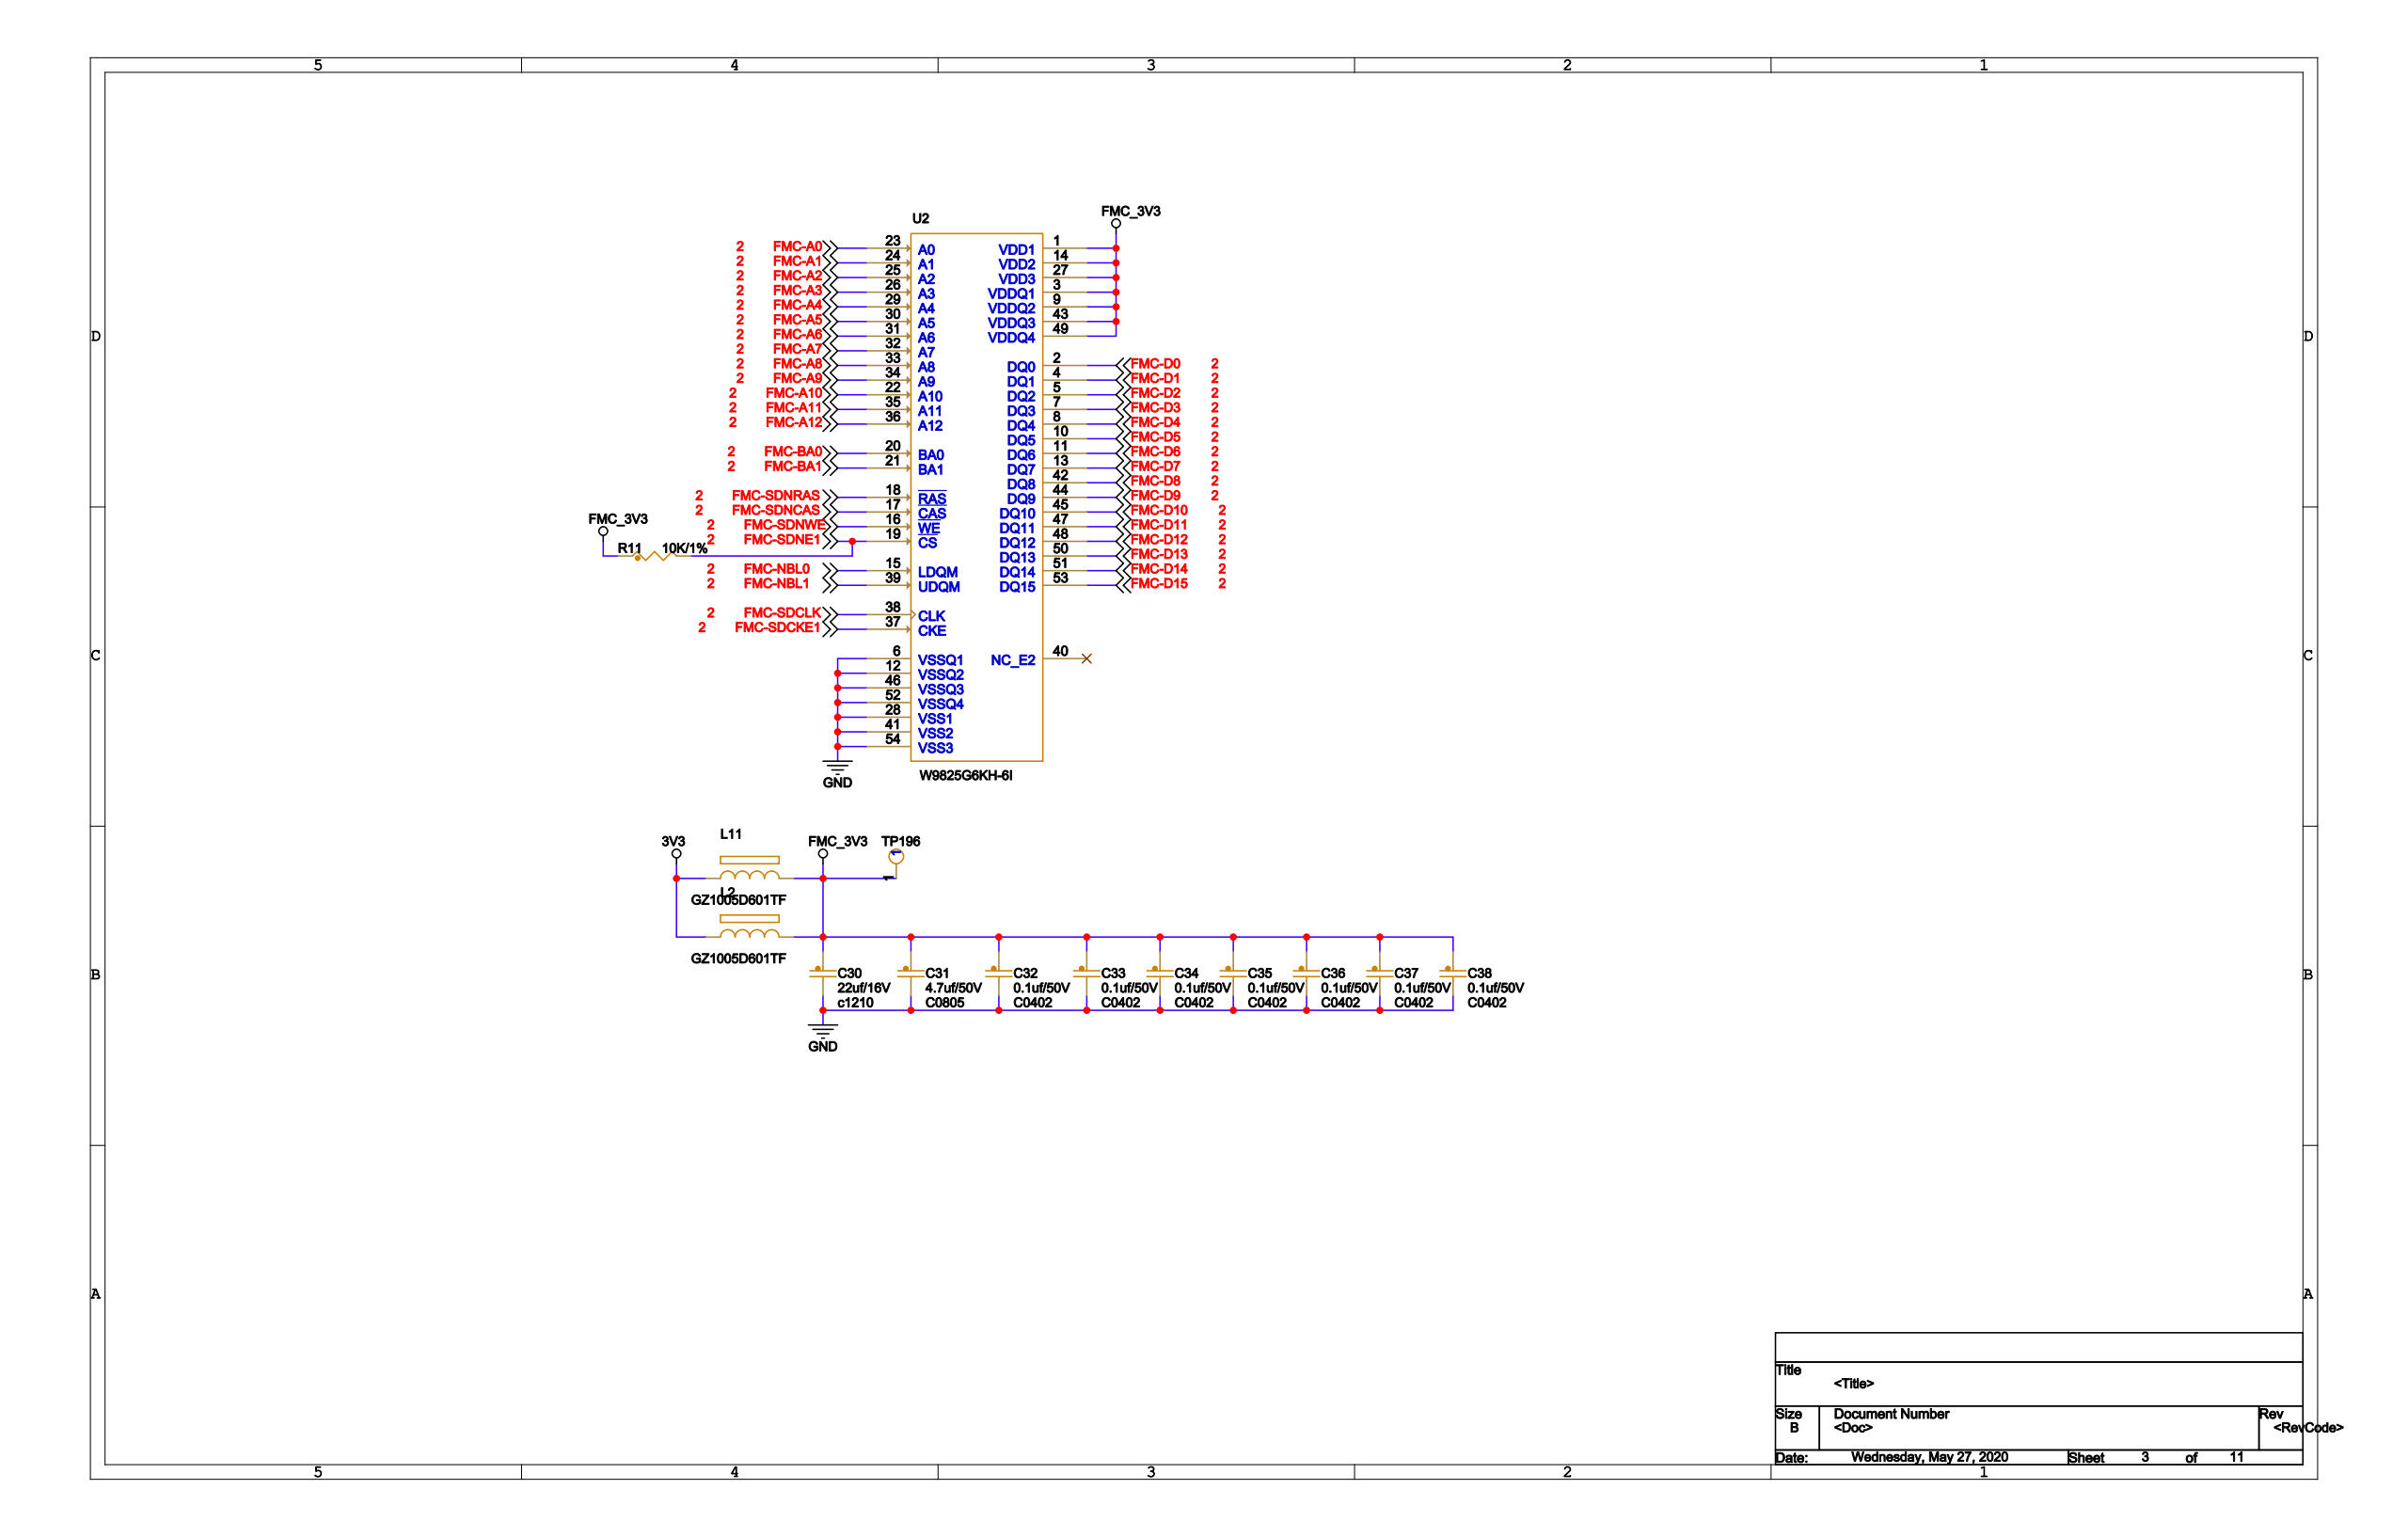Circuit board | Cadence Allegro | 521 parts | 239 nets | one sheet of the schematic
Parts on this sheet (reference | value | footprint):
C30 | 22uf/16V | C1210
C31 | 4.7uf/50V | C0805
C32 | 0.1uf/50V | C0402
C33 | 0.1uf/50V | C0402
C34 | 0.1uf/50V | C0402
C35 | 0.1uf/50V | C0402
C36 | 0.1uf/50V | C0402
C37 | 0.1uf/50V | C0402
C38 | 0.1uf/50V | C0402
L2 | GZ1005D601TF | 0402
L11 | GZ1005D601TF | 0402
R11 | 10K/1% | 0402
TP196 | TESTPOINT | TESTPOINT-33MIL
U2 | W9825G6KH-6I | TSOP54
Nets of these parts (net: part-pin ...):
GND: C30-2 C31-2 C32-2 C33-2 C34-2 C35-2 C36-2 C37-2 C38-2 U2-6 U2-12 U2-28 U2-41 U2-46 U2-52 U2-54
3V3: L2-1 L11-1
FMC_3V3: C30-1 C31-1 C32-1 C33-1 C34-1 C35-1 C36-1 C37-1 C38-1 L2-2 L11-2 R11-1 TP196-1 U2-1 U2-3 U2-9 U2-14 U2-27 U2-43 U2-49
FMC-SDNE1: R11-2 U2-19
FMC-SDNWE: U2-16
FMC-D2: U2-5
FMC-D3: U2-7
FMC-D15: U2-53
FMC-D0: U2-2
FMC-D1: U2-4
FMC-D13: U2-50
FMC-D14: U2-51
FMC-NBL0: U2-15
FMC-NBL1: U2-39
FMC-D7: U2-13
FMC-D8: U2-42
FMC-D9: U2-44
FMC-D10: U2-45
FMC-D11: U2-47
FMC-D12: U2-48
FMC-D4: U2-8
FMC-D5: U2-10
FMC-D6: U2-11
FMC-A0: U2-23
FMC-A1: U2-24
FMC-SDNRAS: U2-18
FMC-A6: U2-31
FMC-A7: U2-32
FMC-A8: U2-33
FMC-A9: U2-34
FMC-A2: U2-25
FMC-A3: U2-26
FMC-A4: U2-29
FMC-A5: U2-30
FMC-A10: U2-22
FMC-A11: U2-35
FMC-SDNCAS: U2-17
FMC-A12: U2-36
FMC-BA0: U2-20
FMC-BA1: U2-21
FMC-SDCLK: U2-38
FMC-SDCKE1: U2-37